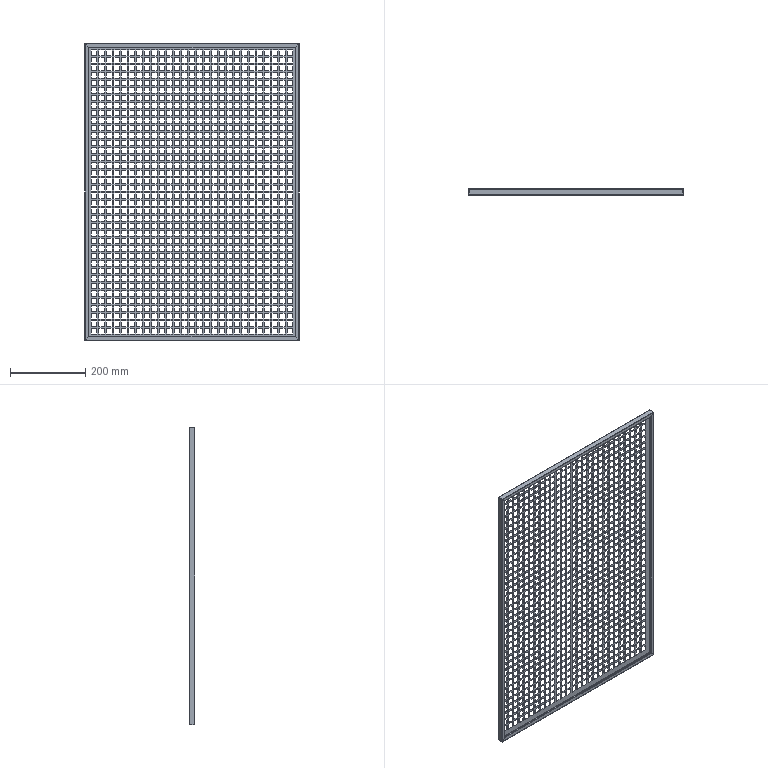Part | STEP file | HESS-408-70-15W-N-21-inner liner partition plate | 1 solid | 4174 faces | volume 280081 mm3 | plane 4142 | cylinder 16 | spline 16 | commonest cylinder face diameters 0.2 x8 2.2 x8